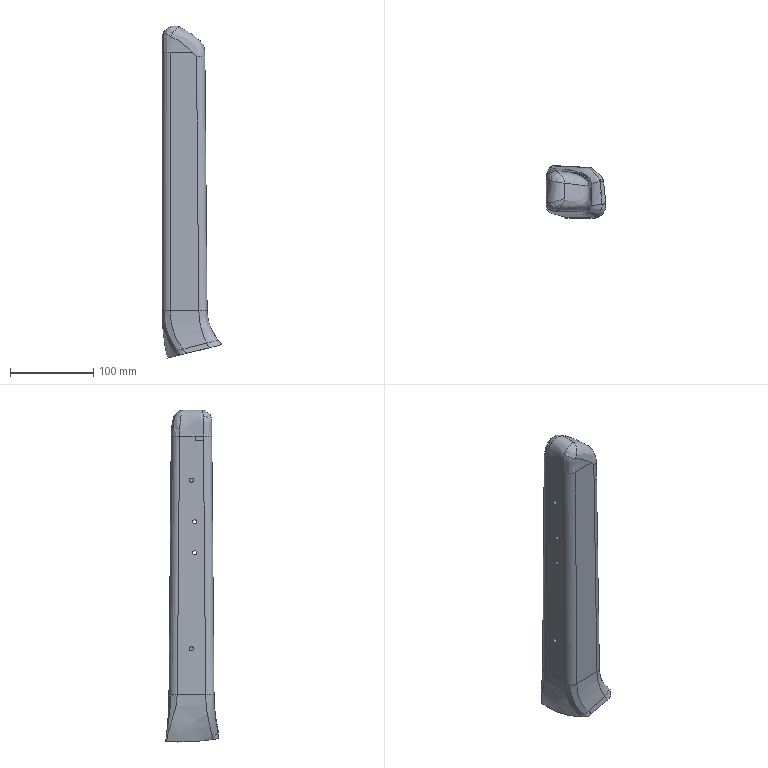Part | STEP file | PN_0006 | 2 solids | 53 faces | box 71.872 x 63.257 x 397.874 mm | volume 548309 mm3 | spline 32 | plane 10 | cylinder 10 | torus 1 | commonest cylinder face diameters 5 x4 20 x3 38.1 x2 7.5 x1